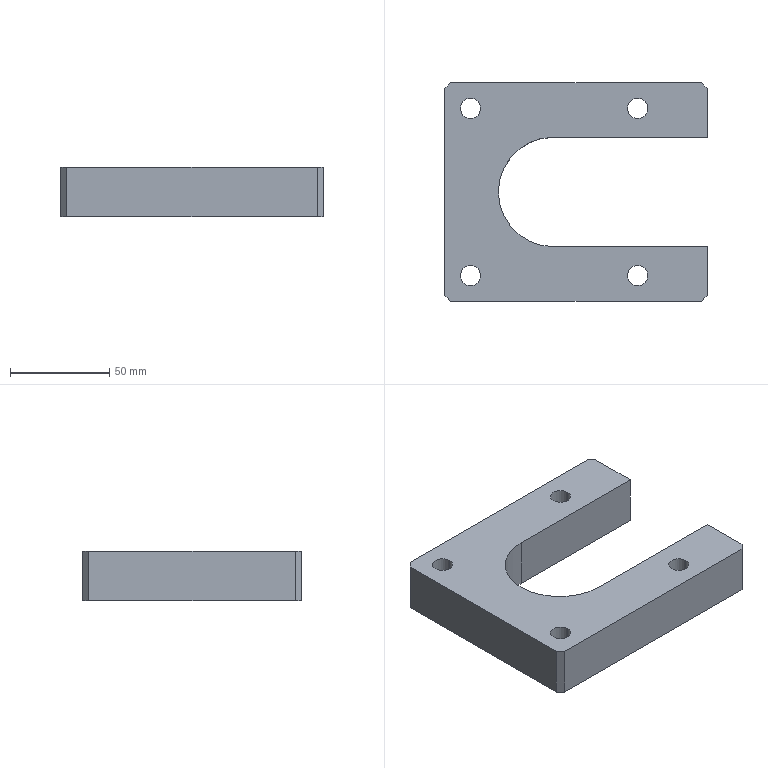Part | STEP file | Bearing mounting plate XG | 1 solid | 23 faces | box 132 x 110 x 25 mm | volume 218118 mm3 | plane 13 | cylinder 10 | commonest cylinder face diameters 10.2 x8 55 x2